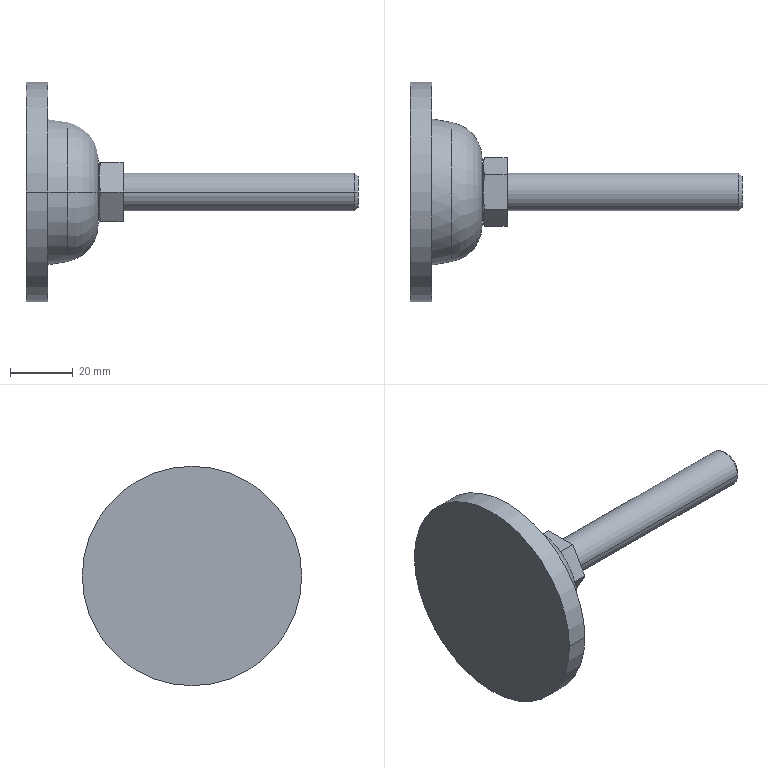Part | STEP file | QA-FJGN12_75pad-1 | 1 solid | 28 faces | box 106 x 70 x 70 mm | volume 59651 mm3 | plane 12 | cylinder 8 | cone 6 | other 2 | commonest cylinder face diameters 12 x2 46.667 x2 64 x2 70 x2